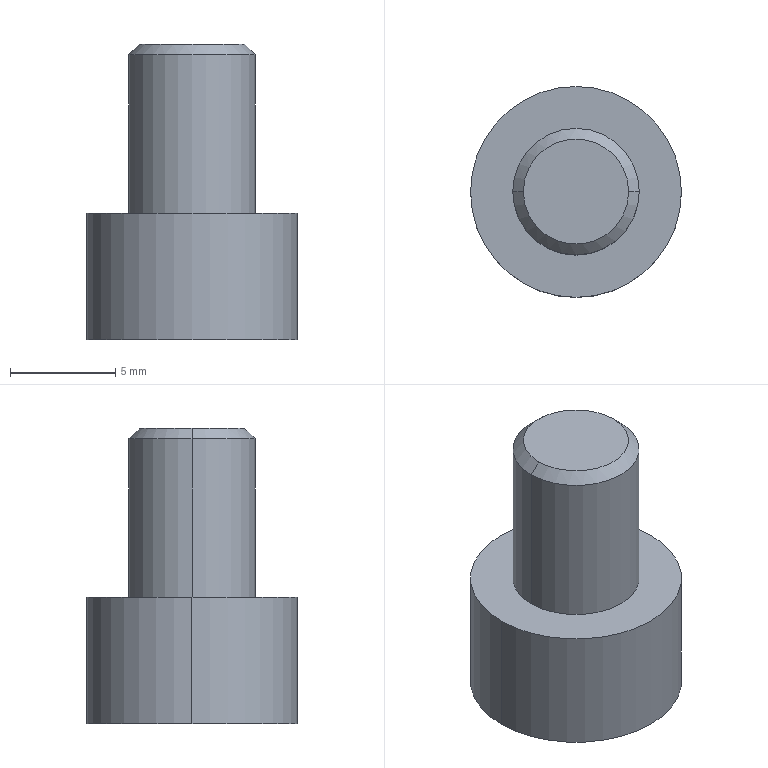Part | STEP file | M6X8 Hex Socket Screw | 1 solid | 22 faces | box 10 x 10 x 14 mm | volume 616.111 mm3 | plane 16 | cylinder 4 | cone 2 | commonest cylinder face diameters 6 x2 10 x2
STEP:
#1=CARTESIAN_POINT('',(0.,0.,0.));
#2=DIRECTION('',(0.,0.,1.));
#3=DIRECTION('',(1.,0.,0.));
#4=AXIS2_PLACEMENT_3D('',#1,#2,#3);
#5=CARTESIAN_POINT('',(2.5,0.,14.));
#6=VERTEX_POINT('',#5);
#7=CARTESIAN_POINT('',(-2.5,0.,14.));
#8=VERTEX_POINT('',#7);
#9=CARTESIAN_POINT('',(0.,0.,14.));
#10=DIRECTION('',(0.,0.,1.));
#11=DIRECTION('',(1.,0.,0.));
#12=AXIS2_PLACEMENT_3D('',#9,#10,#11);
#13=CIRCLE('',#12,2.5);
#14=CARTESIAN_POINT('',(0.,0.,14.));
#15=DIRECTION('',(0.,0.,-1.));
#16=DIRECTION('',(-1.,0.,0.));
#17=AXIS2_PLACEMENT_3D('',#14,#15,#16);
#18=CONICAL_SURFACE('',#17,2.5,0.7854);
#19=CARTESIAN_POINT('',(3.142,0.));
#20=DIRECTION('',(-1.,0.));
#21=VECTOR('',#20,1.);
#22=LINE('',#19,#21);
#23=(GEOMETRIC_REPRESENTATION_CONTEXT(2)PARAMETRIC_REPRESENTATION_CONTEXT()REPRESENTATION_CONTEXT('',''));
#24=DEFINITIONAL_REPRESENTATION('',(#22),#23);
#25=PCURVE('',#18,#24);
#26=CARTESIAN_POINT('',(3.,0.,14.));
#27=DIRECTION('',(0.,0.,1.));
#28=DIRECTION('',(1.,0.,0.));
#29=AXIS2_PLACEMENT_3D('',#26,#27,#28);
#30=PLANE('',#29);
#31=CARTESIAN_POINT('',(-3.,0.));
#32=DIRECTION('',(1.,0.));
#33=AXIS2_PLACEMENT_2D('',#31,#32);
#34=CIRCLE('',#33,2.5);
#35=(GEOMETRIC_REPRESENTATION_CONTEXT(2)PARAMETRIC_REPRESENTATION_CONTEXT()REPRESENTATION_CONTEXT('',''));
#36=DEFINITIONAL_REPRESENTATION('',(#34),#35);
#37=PCURVE('',#30,#36);
#38=SURFACE_CURVE('',#13,(#25,#37),.PCURVE_S1.);
#39=EDGE_CURVE('',#6,#8,#38,.T.);
#40=ORIENTED_EDGE('',*,*,#39,.F.);
#41=CARTESIAN_POINT('',(3.,0.,13.5));
#42=VERTEX_POINT('',#41);
#43=CARTESIAN_POINT('',(2.5,0.,14.));
#44=DIRECTION('',(0.7071,0.,-0.7071));
#45=VECTOR('',#44,1.);
#46=LINE('',#43,#45);
#47=CARTESIAN_POINT('',(3.142,0.));
#48=DIRECTION('',(0.,1.));
#49=VECTOR('',#48,1.);
#50=LINE('',#47,#49);
#51=(GEOMETRIC_REPRESENTATION_CONTEXT(2)PARAMETRIC_REPRESENTATION_CONTEXT()REPRESENTATION_CONTEXT('',''));
#52=DEFINITIONAL_REPRESENTATION('',(#50),#51);
#53=PCURVE('',#18,#52);
#54=CARTESIAN_POINT('',(0.,0.,14.));
#55=DIRECTION('',(0.,0.,-1.));
#56=DIRECTION('',(-1.,0.,0.));
#57=AXIS2_PLACEMENT_3D('',#54,#55,#56);
#58=CONICAL_SURFACE('',#57,2.5,0.7854);
#59=CARTESIAN_POINT('',(3.142,0.));
#60=DIRECTION('',(0.,1.));
#61=VECTOR('',#60,1.);
#62=LINE('',#59,#61);
#63=(GEOMETRIC_REPRESENTATION_CONTEXT(2)PARAMETRIC_REPRESENTATION_CONTEXT()REPRESENTATION_CONTEXT('',''));
#64=DEFINITIONAL_REPRESENTATION('',(#62),#63);
#65=PCURVE('',#58,#64);
#66=SURFACE_CURVE('',#46,(#53,#65),.PCURVE_S1.);
#67=EDGE_CURVE('',#6,#42,#66,.T.);
#68=ORIENTED_EDGE('',*,*,#67,.T.);
#69=CARTESIAN_POINT('',(-3.,0.,13.5));
#70=VERTEX_POINT('',#69);
#71=CARTESIAN_POINT('',(0.,0.,13.5));
#72=DIRECTION('',(0.,0.,-1.));
#73=DIRECTION('',(1.,0.,0.));
#74=AXIS2_PLACEMENT_3D('',#71,#72,#73);
#75=CIRCLE('',#74,3.);
#76=CARTESIAN_POINT('',(-3.142,0.5));
#77=DIRECTION('',(1.,0.));
#78=VECTOR('',#77,1.);
#79=LINE('',#76,#78);
#80=(GEOMETRIC_REPRESENTATION_CONTEXT(2)PARAMETRIC_REPRESENTATION_CONTEXT()REPRESENTATION_CONTEXT('',''));
#81=DEFINITIONAL_REPRESENTATION('',(#79),#80);
#82=PCURVE('',#18,#81);
#83=CARTESIAN_POINT('',(0.,0.,14.));
#84=DIRECTION('',(0.,0.,1.));
#85=DIRECTION('',(1.,0.,0.));
#86=AXIS2_PLACEMENT_3D('',#83,#84,#85);
#87=CYLINDRICAL_SURFACE('',#86,3.);
#88=CARTESIAN_POINT('',(6.283,-0.5));
#89=DIRECTION('',(-1.,0.));
#90=VECTOR('',#89,1.);
#91=LINE('',#88,#90);
#92=(GEOMETRIC_REPRESENTATION_CONTEXT(2)PARAMETRIC_REPRESENTATION_CONTEXT()REPRESENTATION_CONTEXT('',''));
#93=DEFINITIONAL_REPRESENTATION('',(#91),#92);
#94=PCURVE('',#87,#93);
#95=SURFACE_CURVE('',#75,(#82,#94),.PCURVE_S1.);
#96=EDGE_CURVE('',#70,#42,#95,.T.);
#97=ORIENTED_EDGE('',*,*,#96,.F.);
#98=CARTESIAN_POINT('',(-2.5,0.,14.));
#99=DIRECTION('',(-0.7071,0.,-0.7071));
#100=VECTOR('',#99,1.);
#101=LINE('',#98,#100);
#102=CARTESIAN_POINT('',(0.,0.));
#103=DIRECTION('',(0.,1.));
#104=VECTOR('',#103,1.);
#105=LINE('',#102,#104);
#106=(GEOMETRIC_REPRESENTATION_CONTEXT(2)PARAMETRIC_REPRESENTATION_CONTEXT()REPRESENTATION_CONTEXT('',''));
#107=DEFINITIONAL_REPRESENTATION('',(#105),#106);
#108=PCURVE('',#18,#107);
#109=CARTESIAN_POINT('',(6.283,0.));
#110=DIRECTION('',(0.,1.));
#111=VECTOR('',#110,1.);
#112=LINE('',#109,#111);
#113=(GEOMETRIC_REPRESENTATION_CONTEXT(2)PARAMETRIC_REPRESENTATION_CONTEXT()REPRESENTATION_CONTEXT('',''));
#114=DEFINITIONAL_REPRESENTATION('',(#112),#113);
#115=PCURVE('',#58,#114);
#116=SURFACE_CURVE('',#101,(#108,#115),.PCURVE_S1.);
#117=EDGE_CURVE('',#8,#70,#116,.T.);
#118=ORIENTED_EDGE('',*,*,#117,.F.);
#119=EDGE_LOOP('',(#40,#68,#97,#118));
#120=FACE_BOUND('',#119,.T.);
#121=ADVANCED_FACE('',(#120),#18,.T.);
#122=CARTESIAN_POINT('',(3.,0.,6.));
#123=VERTEX_POINT('',#122);
#124=CARTESIAN_POINT('',(-3.,0.,6.));
#125=VERTEX_POINT('',#124);
#126=CARTESIAN_POINT('',(0.,0.,6.));
#127=DIRECTION('',(0.,0.,1.));
#128=DIRECTION('',(1.,0.,0.));
#129=AXIS2_PLACEMENT_3D('',#126,#127,#128);
#130=CIRCLE('',#129,3.);
#131=CARTESIAN_POINT('',(0.,-8.));
#132=DIRECTION('',(1.,0.));
#133=VECTOR('',#132,1.);
#134=LINE('',#131,#133);
#135=(GEOMETRIC_REPRESENTATION_CONTEXT(2)PARAMETRIC_REPRESENTATION_CONTEXT()REPRESENTATION_CONTEXT('',''));
#136=DEFINITIONAL_REPRESENTATION('',(#134),#135);
#137=PCURVE('',#87,#136);
#138=CARTESIAN_POINT('',(5.,0.,6.));
#139=DIRECTION('',(0.,0.,1.));
#140=DIRECTION('',(1.,0.,0.));
#141=AXIS2_PLACEMENT_3D('',#138,#139,#140);
#142=PLANE('',#141);
#143=CARTESIAN_POINT('',(-5.,0.));
#144=DIRECTION('',(1.,0.));
#145=AXIS2_PLACEMENT_2D('',#143,#144);
#146=CIRCLE('',#145,3.);
#147=(GEOMETRIC_REPRESENTATION_CONTEXT(2)PARAMETRIC_REPRESENTATION_CONTEXT()REPRESENTATION_CONTEXT('',''));
#148=DEFINITIONAL_REPRESENTATION('',(#146),#147);
#149=PCURVE('',#142,#148);
#150=SURFACE_CURVE('',#130,(#137,#149),.PCURVE_S1.);
#151=EDGE_CURVE('',#123,#125,#150,.T.);
#152=ORIENTED_EDGE('',*,*,#151,.T.);
#153=CARTESIAN_POINT('',(-3.,0.,14.));
#154=DIRECTION('',(0.,0.,1.));
#155=VECTOR('',#154,1.);
#156=LINE('',#153,#155);
#157=CARTESIAN_POINT('',(3.142,0.));
#158=DIRECTION('',(0.,1.));
#159=VECTOR('',#158,1.);
#160=LINE('',#157,#159);
#161=(GEOMETRIC_REPRESENTATION_CONTEXT(2)PARAMETRIC_REPRESENTATION_CONTEXT()REPRESENTATION_CONTEXT('',''));
#162=DEFINITIONAL_REPRESENTATION('',(#160),#161);
#163=PCURVE('',#87,#162);
#164=CARTESIAN_POINT('',(0.,0.,14.));
#165=DIRECTION('',(0.,0.,1.));
#166=DIRECTION('',(1.,0.,0.));
#167=AXIS2_PLACEMENT_3D('',#164,#165,#166);
#168=CYLINDRICAL_SURFACE('',#167,3.);
#169=CARTESIAN_POINT('',(3.142,0.));
#170=DIRECTION('',(0.,1.));
#171=VECTOR('',#170,1.);
#172=LINE('',#169,#171);
#173=(GEOMETRIC_REPRESENTATION_CONTEXT(2)PARAMETRIC_REPRESENTATION_CONTEXT()REPRESENTATION_CONTEXT('',''));
#174=DEFINITIONAL_REPRESENTATION('',(#172),#173);
#175=PCURVE('',#168,#174);
#176=SURFACE_CURVE('',#156,(#163,#175),.PCURVE_S1.);
#177=EDGE_CURVE('',#125,#70,#176,.T.);
#178=ORIENTED_EDGE('',*,*,#177,.T.);
#179=ORIENTED_EDGE('',*,*,#96,.T.);
#180=CARTESIAN_POINT('',(3.,0.,14.));
#181=DIRECTION('',(0.,0.,1.));
#182=VECTOR('',#181,1.);
#183=LINE('',#180,#182);
#184=CARTESIAN_POINT('',(0.,0.));
#185=DIRECTION('',(0.,1.));
#186=VECTOR('',#185,1.);
#187=LINE('',#184,#186);
#188=(GEOMETRIC_REPRESENTATION_CONTEXT(2)PARAMETRIC_REPRESENTATION_CONTEXT()REPRESENTATION_CONTEXT('',''));
#189=DEFINITIONAL_REPRESENTATION('',(#187),#188);
#190=PCURVE('',#87,#189);
#191=CARTESIAN_POINT('',(6.283,0.));
#192=DIRECTION('',(0.,1.));
#193=VECTOR('',#192,1.);
#194=LINE('',#191,#193);
#195=(GEOMETRIC_REPRESENTATION_CONTEXT(2)PARAMETRIC_REPRESENTATION_CONTEXT()REPRESENTATION_CONTEXT('',''));
#196=DEFINITIONAL_REPRESENTATION('',(#194),#195);
#197=PCURVE('',#168,#196);
#198=SURFACE_CURVE('',#183,(#190,#197),.PCURVE_S1.);
#199=EDGE_CURVE('',#123,#42,#198,.T.);
#200=ORIENTED_EDGE('',*,*,#199,.F.);
#201=EDGE_LOOP('',(#152,#178,#179,#200));
#202=FACE_BOUND('',#201,.T.);
#203=ADVANCED_FACE('',(#202),#87,.T.);
#204=CARTESIAN_POINT('',(5.,0.,0.));
#205=VERTEX_POINT('',#204);
#206=CARTESIAN_POINT('',(-5.,0.,0.));
#207=VERTEX_POINT('',#206);
#208=CARTESIAN_POINT('',(0.,0.,0.));
#209=DIRECTION('',(0.,0.,1.));
#210=DIRECTION('',(1.,0.,0.));
#211=AXIS2_PLACEMENT_3D('',#208,#209,#210);
#212=CIRCLE('',#211,5.);
#213=CARTESIAN_POINT('',(0.,0.,14.));
#214=DIRECTION('',(0.,0.,1.));
#215=DIRECTION('',(1.,0.,0.));
#216=AXIS2_PLACEMENT_3D('',#213,#214,#215);
#217=CYLINDRICAL_SURFACE('',#216,5.);
#218=CARTESIAN_POINT('',(0.,-14.));
#219=DIRECTION('',(1.,0.));
#220=VECTOR('',#219,1.);
#221=LINE('',#218,#220);
#222=(GEOMETRIC_REPRESENTATION_CONTEXT(2)PARAMETRIC_REPRESENTATION_CONTEXT()REPRESENTATION_CONTEXT('',''));
#223=DEFINITIONAL_REPRESENTATION('',(#221),#222);
#224=PCURVE('',#217,#223);
#225=CARTESIAN_POINT('',(0.,0.,0.));
#226=DIRECTION('',(0.,0.,-1.));
#227=DIRECTION('',(-1.,0.,0.));
#228=AXIS2_PLACEMENT_3D('',#225,#226,#227);
#229=PLANE('',#228);
#230=CARTESIAN_POINT('',(-5.,0.));
#231=CARTESIAN_POINT('',(-5.,8.66));
#232=CARTESIAN_POINT('',(2.5,4.33));
#233=CARTESIAN_POINT('',(10.,0.));
#234=CARTESIAN_POINT('',(2.5,-4.33));
#235=CARTESIAN_POINT('',(-5.,-8.66));
#236=CARTESIAN_POINT('',(-5.,0.));
#237=(BOUNDED_CURVE()B_SPLINE_CURVE(2,(#230,#231,#232,#233,#234,#235,#236),.UNSPECIFIED.,.T.,.F.)B_SPLINE_CURVE_WITH_KNOTS((1,2,2,2,2,1),(-2.094,0.,2.094,4.189,6.283,8.378),.UNSPECIFIED.)CURVE()GEOMETRIC_REPRESENTATION_ITEM()RATIONAL_B_SPLINE_CURVE((1.,0.5,1.,0.5,1.,0.5,1.))REPRESENTATION_ITEM(''));
#238=(GEOMETRIC_REPRESENTATION_CONTEXT(2)PARAMETRIC_REPRESENTATION_CONTEXT()REPRESENTATION_CONTEXT('',''));
#239=DEFINITIONAL_REPRESENTATION('',(#237),#238);
#240=PCURVE('',#229,#239);
#241=SURFACE_CURVE('',#212,(#224,#240),.PCURVE_S1.);
#242=EDGE_CURVE('',#205,#207,#241,.T.);
#243=ORIENTED_EDGE('',*,*,#242,.T.);
#244=CARTESIAN_POINT('',(-5.,0.,6.));
#245=VERTEX_POINT('',#244);
#246=CARTESIAN_POINT('',(-5.,0.,14.));
#247=DIRECTION('',(0.,0.,1.));
#248=VECTOR('',#247,1.);
#249=LINE('',#246,#248);
#250=CARTESIAN_POINT('',(3.142,0.));
#251=DIRECTION('',(0.,1.));
#252=VECTOR('',#251,1.);
#253=LINE('',#250,#252);
#254=(GEOMETRIC_REPRESENTATION_CONTEXT(2)PARAMETRIC_REPRESENTATION_CONTEXT()REPRESENTATION_CONTEXT('',''));
#255=DEFINITIONAL_REPRESENTATION('',(#253),#254);
#256=PCURVE('',#217,#255);
#257=CARTESIAN_POINT('',(0.,0.,14.));
#258=DIRECTION('',(0.,0.,1.));
#259=DIRECTION('',(1.,0.,0.));
#260=AXIS2_PLACEMENT_3D('',#257,#258,#259);
#261=CYLINDRICAL_SURFACE('',#260,5.);
#262=CARTESIAN_POINT('',(3.142,0.));
#263=DIRECTION('',(0.,1.));
#264=VECTOR('',#263,1.);
#265=LINE('',#262,#264);
#266=(GEOMETRIC_REPRESENTATION_CONTEXT(2)PARAMETRIC_REPRESENTATION_CONTEXT()REPRESENTATION_CONTEXT('',''));
#267=DEFINITIONAL_REPRESENTATION('',(#265),#266);
#268=PCURVE('',#261,#267);
#269=SURFACE_CURVE('',#249,(#256,#268),.PCURVE_S1.);
#270=EDGE_CURVE('',#207,#245,#269,.T.);
#271=ORIENTED_EDGE('',*,*,#270,.T.);
#272=CARTESIAN_POINT('',(5.,0.,6.));
#273=VERTEX_POINT('',#272);
#274=CARTESIAN_POINT('',(0.,0.,6.));
#275=DIRECTION('',(0.,0.,1.));
#276=DIRECTION('',(1.,0.,0.));
#277=AXIS2_PLACEMENT_3D('',#274,#275,#276);
#278=CIRCLE('',#277,5.);
#279=CARTESIAN_POINT('',(0.,-8.));
#280=DIRECTION('',(1.,0.));
#281=VECTOR('',#280,1.);
#282=LINE('',#279,#281);
#283=(GEOMETRIC_REPRESENTATION_CONTEXT(2)PARAMETRIC_REPRESENTATION_CONTEXT()REPRESENTATION_CONTEXT('',''));
#284=DEFINITIONAL_REPRESENTATION('',(#282),#283);
#285=PCURVE('',#217,#284);
#286=CARTESIAN_POINT('',(-5.,0.));
#287=DIRECTION('',(1.,0.));
#288=AXIS2_PLACEMENT_2D('',#286,#287);
#289=CIRCLE('',#288,5.);
#290=(GEOMETRIC_REPRESENTATION_CONTEXT(2)PARAMETRIC_REPRESENTATION_CONTEXT()REPRESENTATION_CONTEXT('',''));
#291=DEFINITIONAL_REPRESENTATION('',(#289),#290);
#292=PCURVE('',#142,#291);
#293=SURFACE_CURVE('',#278,(#285,#292),.PCURVE_S1.);
#294=EDGE_CURVE('',#273,#245,#293,.T.);
#295=ORIENTED_EDGE('',*,*,#294,.F.);
#296=CARTESIAN_POINT('',(5.,0.,14.));
#297=DIRECTION('',(0.,0.,1.));
#298=VECTOR('',#297,1.);
#299=LINE('',#296,#298);
#300=CARTESIAN_POINT('',(0.,0.));
#301=DIRECTION('',(0.,1.));
#302=VECTOR('',#301,1.);
#303=LINE('',#300,#302);
#304=(GEOMETRIC_REPRESENTATION_CONTEXT(2)PARAMETRIC_REPRESENTATION_CONTEXT()REPRESENTATION_CONTEXT('',''));
#305=DEFINITIONAL_REPRESENTATION('',(#303),#304);
#306=PCURVE('',#217,#305);
#307=CARTESIAN_POINT('',(6.283,0.));
#308=DIRECTION('',(0.,1.));
#309=VECTOR('',#308,1.);
#310=LINE('',#307,#309);
#311=(GEOMETRIC_REPRESENTATION_CONTEXT(2)PARAMETRIC_REPRESENTATION_CONTEXT()REPRESENTATION_CONTEXT('',''));
#312=DEFINITIONAL_REPRESENTATION('',(#310),#311);
#313=PCURVE('',#261,#312);
#314=SURFACE_CURVE('',#299,(#306,#313),.PCURVE_S1.);
#315=EDGE_CURVE('',#205,#273,#314,.T.);
#316=ORIENTED_EDGE('',*,*,#315,.F.);
#317=EDGE_LOOP('',(#243,#271,#295,#316));
#318=FACE_BOUND('',#317,.T.);
#319=ADVANCED_FACE('',(#318),#217,.T.);
#320=CARTESIAN_POINT('',(1.443,-2.5,0.));
#321=VERTEX_POINT('',#320);
#322=CARTESIAN_POINT('',(-1.443,-2.5,0.));
#323=VERTEX_POINT('',#322);
#324=CARTESIAN_POINT('',(1.443,-2.5,0.));
#325=DIRECTION('',(-1.,0.,0.));
#326=VECTOR('',#325,1.);
#327=LINE('',#324,#326);
#328=CARTESIAN_POINT('',(-1.443,-2.5));
#329=DIRECTION('',(1.,0.));
#330=VECTOR('',#329,1.);
#331=LINE('',#328,#330);
#332=(GEOMETRIC_REPRESENTATION_CONTEXT(2)PARAMETRIC_REPRESENTATION_CONTEXT()REPRESENTATION_CONTEXT('',''));
#333=DEFINITIONAL_REPRESENTATION('',(#331),#332);
#334=PCURVE('',#229,#333);
#335=CARTESIAN_POINT('',(1.443,-2.5,4.));
#336=DIRECTION('',(0.,-1.,0.));
#337=DIRECTION('',(1.,0.,0.));
#338=AXIS2_PLACEMENT_3D('',#335,#336,#337);
#339=PLANE('',#338);
#340=CARTESIAN_POINT('',(0.,-4.));
#341=DIRECTION('',(-1.,0.));
#342=VECTOR('',#341,1.);
#343=LINE('',#340,#342);
#344=(GEOMETRIC_REPRESENTATION_CONTEXT(2)PARAMETRIC_REPRESENTATION_CONTEXT()REPRESENTATION_CONTEXT('',''));
#345=DEFINITIONAL_REPRESENTATION('',(#343),#344);
#346=PCURVE('',#339,#345);
#347=SURFACE_CURVE('',#327,(#334,#346),.PCURVE_S1.);
#348=EDGE_CURVE('',#321,#323,#347,.T.);
#349=ORIENTED_EDGE('',*,*,#348,.F.);
#350=CARTESIAN_POINT('',(2.887,0.,0.));
#351=VERTEX_POINT('',#350);
#352=CARTESIAN_POINT('',(2.887,0.,0.));
#353=DIRECTION('',(-0.5,-0.866,0.));
#354=VECTOR('',#353,1.);
#355=LINE('',#352,#354);
#356=CARTESIAN_POINT('',(-2.887,0.));
#357=DIRECTION('',(0.5,-0.866));
#358=VECTOR('',#357,1.);
#359=LINE('',#356,#358);
#360=(GEOMETRIC_REPRESENTATION_CONTEXT(2)PARAMETRIC_REPRESENTATION_CONTEXT()REPRESENTATION_CONTEXT('',''));
#361=DEFINITIONAL_REPRESENTATION('',(#359),#360);
#362=PCURVE('',#229,#361);
#363=CARTESIAN_POINT('',(2.887,0.,4.));
#364=DIRECTION('',(0.866,-0.5,0.));
#365=DIRECTION('',(0.5,0.866,0.));
#366=AXIS2_PLACEMENT_3D('',#363,#364,#365);
#367=PLANE('',#366);
#368=CARTESIAN_POINT('',(0.,-4.));
#369=DIRECTION('',(-1.,0.));
#370=VECTOR('',#369,1.);
#371=LINE('',#368,#370);
#372=(GEOMETRIC_REPRESENTATION_CONTEXT(2)PARAMETRIC_REPRESENTATION_CONTEXT()REPRESENTATION_CONTEXT('',''));
#373=DEFINITIONAL_REPRESENTATION('',(#371),#372);
#374=PCURVE('',#367,#373);
#375=SURFACE_CURVE('',#355,(#362,#374),.PCURVE_S1.);
#376=EDGE_CURVE('',#351,#321,#375,.T.);
#377=ORIENTED_EDGE('',*,*,#376,.F.);
#378=CARTESIAN_POINT('',(1.443,2.5,0.));
#379=VERTEX_POINT('',#378);
#380=CARTESIAN_POINT('',(1.443,2.5,0.));
#381=DIRECTION('',(0.5,-0.866,0.));
#382=VECTOR('',#381,1.);
#383=LINE('',#380,#382);
#384=CARTESIAN_POINT('',(-1.443,2.5));
#385=DIRECTION('',(-0.5,-0.866));
#386=VECTOR('',#385,1.);
#387=LINE('',#384,#386);
#388=(GEOMETRIC_REPRESENTATION_CONTEXT(2)PARAMETRIC_REPRESENTATION_CONTEXT()REPRESENTATION_CONTEXT('',''));
#389=DEFINITIONAL_REPRESENTATION('',(#387),#388);
#390=PCURVE('',#229,#389);
#391=CARTESIAN_POINT('',(1.443,2.5,4.));
#392=DIRECTION('',(0.866,0.5,0.));
#393=DIRECTION('',(-0.5,0.866,0.));
#394=AXIS2_PLACEMENT_3D('',#391,#392,#393);
#395=PLANE('',#394);
#396=CARTESIAN_POINT('',(0.,-4.));
#397=DIRECTION('',(-1.,0.));
#398=VECTOR('',#397,1.);
#399=LINE('',#396,#398);
#400=(GEOMETRIC_REPRESENTATION_CONTEXT(2)PARAMETRIC_REPRESENTATION_CONTEXT()REPRESENTATION_CONTEXT('',''));
#401=DEFINITIONAL_REPRESENTATION('',(#399),#400);
#402=PCURVE('',#395,#401);
#403=SURFACE_CURVE('',#383,(#390,#402),.PCURVE_S1.);
#404=EDGE_CURVE('',#379,#351,#403,.T.);
#405=ORIENTED_EDGE('',*,*,#404,.F.);
#406=CARTESIAN_POINT('',(-1.443,2.5,0.));
#407=VERTEX_POINT('',#406);
#408=CARTESIAN_POINT('',(-1.443,2.5,0.));
#409=DIRECTION('',(1.,0.,0.));
#410=VECTOR('',#409,1.);
#411=LINE('',#408,#410);
#412=CARTESIAN_POINT('',(1.443,2.5));
#413=DIRECTION('',(-1.,0.));
#414=VECTOR('',#413,1.);
#415=LINE('',#412,#414);
#416=(GEOMETRIC_REPRESENTATION_CONTEXT(2)PARAMETRIC_REPRESENTATION_CONTEXT()REPRESENTATION_CONTEXT('',''));
#417=DEFINITIONAL_REPRESENTATION('',(#415),#416);
#418=PCURVE('',#229,#417);
#419=CARTESIAN_POINT('',(-1.443,2.5,4.));
#420=DIRECTION('',(0.,1.,0.));
#421=DIRECTION('',(-1.,0.,0.));
#422=AXIS2_PLACEMENT_3D('',#419,#420,#421);
#423=PLANE('',#422);
#424=CARTESIAN_POINT('',(0.,-4.));
#425=DIRECTION('',(-1.,0.));
#426=VECTOR('',#425,1.);
#427=LINE('',#424,#426);
#428=(GEOMETRIC_REPRESENTATION_CONTEXT(2)PARAMETRIC_REPRESENTATION_CONTEXT()REPRESENTATION_CONTEXT('',''));
#429=DEFINITIONAL_REPRESENTATION('',(#427),#428);
#430=PCURVE('',#423,#429);
#431=SURFACE_CURVE('',#411,(#418,#430),.PCURVE_S1.);
#432=EDGE_CURVE('',#407,#379,#431,.T.);
#433=ORIENTED_EDGE('',*,*,#432,.F.);
#434=CARTESIAN_POINT('',(-2.887,0.,0.));
#435=VERTEX_POINT('',#434);
#436=CARTESIAN_POINT('',(-2.887,0.,0.));
#437=DIRECTION('',(0.5,0.866,0.));
#438=VECTOR('',#437,1.);
#439=LINE('',#436,#438);
#440=CARTESIAN_POINT('',(2.887,0.));
#441=DIRECTION('',(-0.5,0.866));
#442=VECTOR('',#441,1.);
#443=LINE('',#440,#442);
#444=(GEOMETRIC_REPRESENTATION_CONTEXT(2)PARAMETRIC_REPRESENTATION_CONTEXT()REPRESENTATION_CONTEXT('',''));
#445=DEFINITIONAL_REPRESENTATION('',(#443),#444);
#446=PCURVE('',#229,#445);
#447=CARTESIAN_POINT('',(-2.887,0.,4.));
#448=DIRECTION('',(-0.866,0.5,0.));
#449=DIRECTION('',(-0.5,-0.866,0.));
#450=AXIS2_PLACEMENT_3D('',#447,#448,#449);
#451=PLANE('',#450);
#452=CARTESIAN_POINT('',(0.,-4.));
#453=DIRECTION('',(-1.,0.));
#454=VECTOR('',#453,1.);
#455=LINE('',#452,#454);
#456=(GEOMETRIC_REPRESENTATION_CONTEXT(2)PARAMETRIC_REPRESENTATION_CONTEXT()REPRESENTATION_CONTEXT('',''));
#457=DEFINITIONAL_REPRESENTATION('',(#455),#456);
#458=PCURVE('',#451,#457);
#459=SURFACE_CURVE('',#439,(#446,#458),.PCURVE_S1.);
#460=EDGE_CURVE('',#435,#407,#459,.T.);
#461=ORIENTED_EDGE('',*,*,#460,.F.);
#462=CARTESIAN_POINT('',(-1.443,-2.5,0.));
#463=DIRECTION('',(-0.5,0.866,0.));
#464=VECTOR('',#463,1.);
#465=LINE('',#462,#464);
#466=CARTESIAN_POINT('',(1.443,-2.5));
#467=DIRECTION('',(0.5,0.866));
#468=VECTOR('',#467,1.);
#469=LINE('',#466,#468);
#470=(GEOMETRIC_REPRESENTATION_CONTEXT(2)PARAMETRIC_REPRESENTATION_CONTEXT()REPRESENTATION_CONTEXT('',''));
#471=DEFINITIONAL_REPRESENTATION('',(#469),#470);
#472=PCURVE('',#229,#471);
#473=CARTESIAN_POINT('',(-1.443,-2.5,4.));
#474=DIRECTION('',(-0.866,-0.5,0.));
#475=DIRECTION('',(0.5,-0.866,0.));
#476=AXIS2_PLACEMENT_3D('',#473,#474,#475);
#477=PLANE('',#476);
#478=CARTESIAN_POINT('',(0.,-4.));
#479=DIRECTION('',(-1.,0.));
#480=VECTOR('',#479,1.);
#481=LINE('',#478,#480);
#482=(GEOMETRIC_REPRESENTATION_CONTEXT(2)PARAMETRIC_REPRESENTATION_CONTEXT()REPRESENTATION_CONTEXT('',''));
#483=DEFINITIONAL_REPRESENTATION('',(#481),#482);
#484=PCURVE('',#477,#483);
#485=SURFACE_CURVE('',#465,(#472,#484),.PCURVE_S1.);
#486=EDGE_CURVE('',#323,#435,#485,.T.);
#487=ORIENTED_EDGE('',*,*,#486,.F.);
#488=EDGE_LOOP('',(#349,#377,#405,#433,#461,#487));
#489=FACE_BOUND('',#488,.T.);
#490=ORIENTED_EDGE('',*,*,#242,.F.);
#491=CARTESIAN_POINT('',(0.,0.,0.));
#492=DIRECTION('',(0.,0.,1.));
#493=DIRECTION('',(1.,0.,0.));
#494=AXIS2_PLACEMENT_3D('',#491,#492,#493);
#495=CIRCLE('',#494,5.);
#496=CARTESIAN_POINT('',(-5.,0.));
#497=CARTESIAN_POINT('',(-5.,8.66));
#498=CARTESIAN_POINT('',(2.5,4.33));
#499=CARTESIAN_POINT('',(10.,0.));
#500=CARTESIAN_POINT('',(2.5,-4.33));
#501=CARTESIAN_POINT('',(-5.,-8.66));
#502=CARTESIAN_POINT('',(-5.,0.));
#503=(BOUNDED_CURVE()B_SPLINE_CURVE(2,(#496,#497,#498,#499,#500,#501,#502),.UNSPECIFIED.,.T.,.F.)B_SPLINE_CURVE_WITH_KNOTS((1,2,2,2,2,1),(-2.094,0.,2.094,4.189,6.283,8.378),.UNSPECIFIED.)CURVE()GEOMETRIC_REPRESENTATION_ITEM()RATIONAL_B_SPLINE_CURVE((1.,0.5,1.,0.5,1.,0.5,1.))REPRESENTATION_ITEM(''));
#504=(GEOMETRIC_REPRESENTATION_CONTEXT(2)PARAMETRIC_REPRESENTATION_CONTEXT()REPRESENTATION_CONTEXT('',''));
#505=DEFINITIONAL_REPRESENTATION('',(#503),#504);
#506=PCURVE('',#229,#505);
#507=CARTESIAN_POINT('',(0.,-14.));
#508=DIRECTION('',(1.,0.));
#509=VECTOR('',#508,1.);
#510=LINE('',#507,#509);
#511=(GEOMETRIC_REPRESENTATION_CONTEXT(2)PARAMETRIC_REPRESENTATION_CONTEXT()REPRESENTATION_CONTEXT('',''));
#512=DEFINITIONAL_REPRESENTATION('',(#510),#511);
#513=PCURVE('',#261,#512);
#514=SURFACE_CURVE('',#495,(#506,#513),.PCURVE_S1.);
#515=EDGE_CURVE('',#207,#205,#514,.T.);
#516=ORIENTED_EDGE('',*,*,#515,.F.);
#517=EDGE_LOOP('',(#490,#516));
#518=FACE_BOUND('',#517,.T.);
#519=ADVANCED_FACE('',(#489,#518),#229,.T.);
#520=ORIENTED_EDGE('',*,*,#270,.F.);
#521=ORIENTED_EDGE('',*,*,#515,.T.);
#522=ORIENTED_EDGE('',*,*,#315,.T.);
#523=CARTESIAN_POINT('',(0.,0.,6.));
#524=DIRECTION('',(0.,0.,1.));
#525=DIRECTION('',(1.,0.,0.));
#526=AXIS2_PLACEMENT_3D('',#523,#524,#525);
#527=CIRCLE('',#526,5.);
#528=CARTESIAN_POINT('',(0.,-8.));
#529=DIRECTION('',(1.,0.));
#530=VECTOR('',#529,1.);
#531=LINE('',#528,#530);
#532=(GEOMETRIC_REPRESENTATION_CONTEXT(2)PARAMETRIC_REPRESENTATION_CONTEXT()REPRESENTATION_CONTEXT('',''));
#533=DEFINITIONAL_REPRESENTATION('',(#531),#532);
#534=PCURVE('',#261,#533);
#535=CARTESIAN_POINT('',(-5.,0.));
#536=DIRECTION('',(1.,0.));
#537=AXIS2_PLACEMENT_2D('',#535,#536);
#538=CIRCLE('',#537,5.);
#539=(GEOMETRIC_REPRESENTATION_CONTEXT(2)PARAMETRIC_REPRESENTATION_CONTEXT()REPRESENTATION_CONTEXT('',''));
#540=DEFINITIONAL_REPRESENTATION('',(#538),#539);
#541=PCURVE('',#142,#540);
#542=SURFACE_CURVE('',#527,(#534,#541),.PCURVE_S1.);
#543=EDGE_CURVE('',#245,#273,#542,.T.);
#544=ORIENTED_EDGE('',*,*,#543,.F.);
#545=EDGE_LOOP('',(#520,#521,#522,#544));
#546=FACE_BOUND('',#545,.T.);
#547=ADVANCED_FACE('',(#546),#261,.T.);
#548=ORIENTED_EDGE('',*,*,#294,.T.);
#549=ORIENTED_EDGE('',*,*,#543,.T.);
#550=EDGE_LOOP('',(#548,#549));
#551=FACE_BOUND('',#550,.T.);
#552=ORIENTED_EDGE('',*,*,#151,.F.);
#553=CARTESIAN_POINT('',(0.,0.,6.));
#554=DIRECTION('',(0.,0.,1.));
#555=DIRECTION('',(1.,0.,0.));
#556=AXIS2_PLACEMENT_3D('',#553,#554,#555);
#557=CIRCLE('',#556,3.);
#558=CARTESIAN_POINT('',(-5.,0.));
#559=DIRECTION('',(1.,0.));
#560=AXIS2_PLACEMENT_2D('',#558,#559);
#561=CIRCLE('',#560,3.);
#562=(GEOMETRIC_REPRESENTATION_CONTEXT(2)PARAMETRIC_REPRESENTATION_CONTEXT()REPRESENTATION_CONTEXT('',''));
#563=DEFINITIONAL_REPRESENTATION('',(#561),#562);
#564=PCURVE('',#142,#563);
#565=CARTESIAN_POINT('',(0.,-8.));
#566=DIRECTION('',(1.,0.));
#567=VECTOR('',#566,1.);
#568=LINE('',#565,#567);
#569=(GEOMETRIC_REPRESENTATION_CONTEXT(2)PARAMETRIC_REPRESENTATION_CONTEXT()REPRESENTATION_CONTEXT('',''));
#570=DEFINITIONAL_REPRESENTATION('',(#568),#569);
#571=PCURVE('',#168,#570);
#572=SURFACE_CURVE('',#557,(#564,#571),.PCURVE_S1.);
#573=EDGE_CURVE('',#125,#123,#572,.T.);
#574=ORIENTED_EDGE('',*,*,#573,.F.);
#575=EDGE_LOOP('',(#552,#574));
#576=FACE_BOUND('',#575,.T.);
#577=ADVANCED_FACE('',(#551,#576),#142,.T.);
#578=ORIENTED_EDGE('',*,*,#177,.F.);
#579=ORIENTED_EDGE('',*,*,#573,.T.);
#580=ORIENTED_EDGE('',*,*,#199,.T.);
#581=CARTESIAN_POINT('',(0.,0.,13.5));
#582=DIRECTION('',(0.,0.,-1.));
#583=DIRECTION('',(1.,0.,0.));
#584=AXIS2_PLACEMENT_3D('',#581,#582,#583);
#585=CIRCLE('',#584,3.);
#586=CARTESIAN_POINT('',(6.283,-0.5));
#587=DIRECTION('',(-1.,0.));
#588=VECTOR('',#587,1.);
#589=LINE('',#586,#588);
#590=(GEOMETRIC_REPRESENTATION_CONTEXT(2)PARAMETRIC_REPRESENTATION_CONTEXT()REPRESENTATION_CONTEXT('',''));
#591=DEFINITIONAL_REPRESENTATION('',(#589),#590);
#592=PCURVE('',#168,#591);
#593=CARTESIAN_POINT('',(3.142,0.5));
#594=DIRECTION('',(1.,0.));
#595=VECTOR('',#594,1.);
#596=LINE('',#593,#595);
#597=(GEOMETRIC_REPRESENTATION_CONTEXT(2)PARAMETRIC_REPRESENTATION_CONTEXT()REPRESENTATION_CONTEXT('',''));
#598=DEFINITIONAL_REPRESENTATION('',(#596),#597);
#599=PCURVE('',#58,#598);
#600=SURFACE_CURVE('',#585,(#592,#599),.PCURVE_S1.);
#601=EDGE_CURVE('',#42,#70,#600,.T.);
#602=ORIENTED_EDGE('',*,*,#601,.T.);
#603=EDGE_LOOP('',(#578,#579,#580,#602));
#604=FACE_BOUND('',#603,.T.);
#605=ADVANCED_FACE('',(#604),#168,.T.);
#606=CARTESIAN_POINT('',(0.,0.,14.));
#607=DIRECTION('',(0.,0.,1.));
#608=DIRECTION('',(1.,0.,0.));
#609=AXIS2_PLACEMENT_3D('',#606,#607,#608);
#610=CIRCLE('',#609,2.5);
#611=CARTESIAN_POINT('',(-3.,0.));
#612=DIRECTION('',(1.,0.));
#613=AXIS2_PLACEMENT_2D('',#611,#612);
#614=CIRCLE('',#613,2.5);
#615=(GEOMETRIC_REPRESENTATION_CONTEXT(2)PARAMETRIC_REPRESENTATION_CONTEXT()REPRESENTATION_CONTEXT('',''));
#616=DEFINITIONAL_REPRESENTATION('',(#614),#615);
#617=PCURVE('',#30,#616);
#618=CARTESIAN_POINT('',(9.425,0.));
#619=DIRECTION('',(-1.,0.));
#620=VECTOR('',#619,1.);
#621=LINE('',#618,#620);
#622=(GEOMETRIC_REPRESENTATION_CONTEXT(2)PARAMETRIC_REPRESENTATION_CONTEXT()REPRESENTATION_CONTEXT('',''));
#623=DEFINITIONAL_REPRESENTATION('',(#621),#622);
#624=PCURVE('',#58,#623);
#625=SURFACE_CURVE('',#610,(#617,#624),.PCURVE_S1.);
#626=EDGE_CURVE('',#8,#6,#625,.T.);
#627=ORIENTED_EDGE('',*,*,#626,.T.);
#628=ORIENTED_EDGE('',*,*,#39,.T.);
#629=EDGE_LOOP('',(#627,#628));
#630=FACE_BOUND('',#629,.T.);
#631=ADVANCED_FACE('',(#630),#30,.T.);
#632=CARTESIAN_POINT('',(-1.443,-2.5,3.));
#633=VERTEX_POINT('',#632);
#634=CARTESIAN_POINT('',(-1.443,-2.5,4.));
#635=DIRECTION('',(0.,0.,-1.));
#636=VECTOR('',#635,1.);
#637=LINE('',#634,#636);
#638=CARTESIAN_POINT('',(-2.887,0.));
#639=DIRECTION('',(0.,-1.));
#640=VECTOR('',#639,1.);
#641=LINE('',#638,#640);
#642=(GEOMETRIC_REPRESENTATION_CONTEXT(2)PARAMETRIC_REPRESENTATION_CONTEXT()REPRESENTATION_CONTEXT('',''));
#643=DEFINITIONAL_REPRESENTATION('',(#641),#642);
#644=PCURVE('',#339,#643);
#645=CARTESIAN_POINT('',(0.,0.));
#646=DIRECTION('',(0.,-1.));
#647=VECTOR('',#646,1.);
#648=LINE('',#645,#647);
#649=(GEOMETRIC_REPRESENTATION_CONTEXT(2)PARAMETRIC_REPRESENTATION_CONTEXT()REPRESENTATION_CONTEXT('',''));
#650=DEFINITIONAL_REPRESENTATION('',(#648),#649);
#651=PCURVE('',#477,#650);
#652=SURFACE_CURVE('',#637,(#644,#651),.PCURVE_S1.);
#653=EDGE_CURVE('',#633,#323,#652,.T.);
#654=ORIENTED_EDGE('',*,*,#653,.F.);
#655=CARTESIAN_POINT('',(1.443,-2.5,3.));
#656=VERTEX_POINT('',#655);
#657=CARTESIAN_POINT('',(1.443,-2.5,3.));
#658=DIRECTION('',(1.,0.,0.));
#659=VECTOR('',#658,1.);
#660=LINE('',#657,#659);
#661=CARTESIAN_POINT('',(0.,-1.));
#662=DIRECTION('',(1.,0.));
#663=VECTOR('',#662,1.);
#664=LINE('',#661,#663);
#665=(GEOMETRIC_REPRESENTATION_CONTEXT(2)PARAMETRIC_REPRESENTATION_CONTEXT()REPRESENTATION_CONTEXT('',''));
#666=DEFINITIONAL_REPRESENTATION('',(#664),#665);
#667=PCURVE('',#339,#666);
#668=CARTESIAN_POINT('',(0.,-1.5,4.));
#669=DIRECTION('',(0.,-0.7071,0.7071));
#670=DIRECTION('',(-1.,0.,0.));
#671=AXIS2_PLACEMENT_3D('',#668,#669,#670);
#672=PLANE('',#671);
#673=CARTESIAN_POINT('',(-1.443,1.414));
#674=DIRECTION('',(-1.,0.));
#675=VECTOR('',#674,1.);
#676=LINE('',#673,#675);
#677=(GEOMETRIC_REPRESENTATION_CONTEXT(2)PARAMETRIC_REPRESENTATION_CONTEXT()REPRESENTATION_CONTEXT('',''));
#678=DEFINITIONAL_REPRESENTATION('',(#676),#677);
#679=PCURVE('',#672,#678);
#680=SURFACE_CURVE('',#660,(#667,#679),.PCURVE_S1.);
#681=EDGE_CURVE('',#633,#656,#680,.T.);
#682=ORIENTED_EDGE('',*,*,#681,.T.);
#683=CARTESIAN_POINT('',(1.443,-2.5,4.));
#684=DIRECTION('',(0.,0.,-1.));
#685=VECTOR('',#684,1.);
#686=LINE('',#683,#685);
#687=CARTESIAN_POINT('',(0.,0.));
#688=DIRECTION('',(0.,-1.));
#689=VECTOR('',#688,1.);
#690=LINE('',#687,#689);
#691=(GEOMETRIC_REPRESENTATION_CONTEXT(2)PARAMETRIC_REPRESENTATION_CONTEXT()REPRESENTATION_CONTEXT('',''));
#692=DEFINITIONAL_REPRESENTATION('',(#690),#691);
#693=PCURVE('',#339,#692);
#694=CARTESIAN_POINT('',(-2.887,0.));
#695=DIRECTION('',(0.,-1.));
#696=VECTOR('',#695,1.);
#697=LINE('',#694,#696);
#698=(GEOMETRIC_REPRESENTATION_CONTEXT(2)PARAMETRIC_REPRESENTATION_CONTEXT()REPRESENTATION_CONTEXT('',''));
#699=DEFINITIONAL_REPRESENTATION('',(#697),#698);
#700=PCURVE('',#367,#699);
#701=SURFACE_CURVE('',#686,(#693,#700),.PCURVE_S1.);
#702=EDGE_CURVE('',#656,#321,#701,.T.);
#703=ORIENTED_EDGE('',*,*,#702,.T.);
#704=ORIENTED_EDGE('',*,*,#348,.T.);
#705=EDGE_LOOP('',(#654,#682,#703,#704));
#706=FACE_BOUND('',#705,.T.);
#707=ADVANCED_FACE('',(#706),#339,.F.);
#708=ORIENTED_EDGE('',*,*,#702,.F.);
#709=CARTESIAN_POINT('',(2.887,0.,3.));
#710=VERTEX_POINT('',#709);
#711=CARTESIAN_POINT('',(2.887,0.,3.));
#712=DIRECTION('',(0.5,0.866,0.));
#713=VECTOR('',#712,1.);
#714=LINE('',#711,#713);
#715=CARTESIAN_POINT('',(0.,-1.));
#716=DIRECTION('',(1.,0.));
#717=VECTOR('',#716,1.);
#718=LINE('',#715,#717);
#719=(GEOMETRIC_REPRESENTATION_CONTEXT(2)PARAMETRIC_REPRESENTATION_CONTEXT()REPRESENTATION_CONTEXT('',''));
#720=DEFINITIONAL_REPRESENTATION('',(#718),#719);
#721=PCURVE('',#367,#720);
#722=CARTESIAN_POINT('',(1.299,-0.75,4.));
#723=DIRECTION('',(0.6124,-0.3536,0.7071));
#724=DIRECTION('',(-0.5,-0.866,0.));
#725=AXIS2_PLACEMENT_3D('',#722,#723,#724);
#726=PLANE('',#725);
#727=CARTESIAN_POINT('',(-1.443,1.414));
#728=DIRECTION('',(-1.,0.));
#729=VECTOR('',#728,1.);
#730=LINE('',#727,#729);
#731=(GEOMETRIC_REPRESENTATION_CONTEXT(2)PARAMETRIC_REPRESENTATION_CONTEXT()REPRESENTATION_CONTEXT('',''));
#732=DEFINITIONAL_REPRESENTATION('',(#730),#731);
#733=PCURVE('',#726,#732);
#734=SURFACE_CURVE('',#714,(#721,#733),.PCURVE_S1.);
#735=EDGE_CURVE('',#656,#710,#734,.T.);
#736=ORIENTED_EDGE('',*,*,#735,.T.);
#737=CARTESIAN_POINT('',(2.887,0.,4.));
#738=DIRECTION('',(0.,0.,-1.));
#739=VECTOR('',#738,1.);
#740=LINE('',#737,#739);
#741=CARTESIAN_POINT('',(0.,0.));
#742=DIRECTION('',(0.,-1.));
#743=VECTOR('',#742,1.);
#744=LINE('',#741,#743);
#745=(GEOMETRIC_REPRESENTATION_CONTEXT(2)PARAMETRIC_REPRESENTATION_CONTEXT()REPRESENTATION_CONTEXT('',''));
#746=DEFINITIONAL_REPRESENTATION('',(#744),#745);
#747=PCURVE('',#367,#746);
#748=CARTESIAN_POINT('',(-2.887,0.));
#749=DIRECTION('',(0.,-1.));
#750=VECTOR('',#749,1.);
#751=LINE('',#748,#750);
#752=(GEOMETRIC_REPRESENTATION_CONTEXT(2)PARAMETRIC_REPRESENTATION_CONTEXT()REPRESENTATION_CONTEXT('',''));
#753=DEFINITIONAL_REPRESENTATION('',(#751),#752);
#754=PCURVE('',#395,#753);
#755=SURFACE_CURVE('',#740,(#747,#754),.PCURVE_S1.);
#756=EDGE_CURVE('',#710,#351,#755,.T.);
#757=ORIENTED_EDGE('',*,*,#756,.T.);
#758=ORIENTED_EDGE('',*,*,#376,.T.);
#759=EDGE_LOOP('',(#708,#736,#757,#758));
#760=FACE_BOUND('',#759,.T.);
#761=ADVANCED_FACE('',(#760),#367,.F.);
#762=ORIENTED_EDGE('',*,*,#756,.F.);
#763=CARTESIAN_POINT('',(1.443,2.5,3.));
#764=VERTEX_POINT('',#763);
#765=CARTESIAN_POINT('',(1.443,2.5,3.));
#766=DIRECTION('',(-0.5,0.866,0.));
#767=VECTOR('',#766,1.);
#768=LINE('',#765,#767);
#769=CARTESIAN_POINT('',(0.,-1.));
#770=DIRECTION('',(1.,0.));
#771=VECTOR('',#770,1.);
#772=LINE('',#769,#771);
#773=(GEOMETRIC_REPRESENTATION_CONTEXT(2)PARAMETRIC_REPRESENTATION_CONTEXT()REPRESENTATION_CONTEXT('',''));
#774=DEFINITIONAL_REPRESENTATION('',(#772),#773);
#775=PCURVE('',#395,#774);
#776=CARTESIAN_POINT('',(1.299,0.75,4.));
#777=DIRECTION('',(0.6124,0.3536,0.7071));
#778=DIRECTION('',(0.5,-0.866,0.));
#779=AXIS2_PLACEMENT_3D('',#776,#777,#778);
#780=PLANE('',#779);
#781=CARTESIAN_POINT('',(-1.443,1.414));
#782=DIRECTION('',(-1.,0.));
#783=VECTOR('',#782,1.);
#784=LINE('',#781,#783);
#785=(GEOMETRIC_REPRESENTATION_CONTEXT(2)PARAMETRIC_REPRESENTATION_CONTEXT()REPRESENTATION_CONTEXT('',''));
#786=DEFINITIONAL_REPRESENTATION('',(#784),#785);
#787=PCURVE('',#780,#786);
#788=SURFACE_CURVE('',#768,(#775,#787),.PCURVE_S1.);
#789=EDGE_CURVE('',#710,#764,#788,.T.);
#790=ORIENTED_EDGE('',*,*,#789,.T.);
#791=CARTESIAN_POINT('',(1.443,2.5,4.));
#792=DIRECTION('',(0.,0.,-1.));
#793=VECTOR('',#792,1.);
#794=LINE('',#791,#793);
#795=CARTESIAN_POINT('',(0.,0.));
#796=DIRECTION('',(0.,-1.));
#797=VECTOR('',#796,1.);
#798=LINE('',#795,#797);
#799=(GEOMETRIC_REPRESENTATION_CONTEXT(2)PARAMETRIC_REPRESENTATION_CONTEXT()REPRESENTATION_CONTEXT('',''));
#800=DEFINITIONAL_REPRESENTATION('',(#798),#799);
#801=PCURVE('',#395,#800);
#802=CARTESIAN_POINT('',(-2.887,0.));
#803=DIRECTION('',(0.,-1.));
#804=VECTOR('',#803,1.);
#805=LINE('',#802,#804);
#806=(GEOMETRIC_REPRESENTATION_CONTEXT(2)PARAMETRIC_REPRESENTATION_CONTEXT()REPRESENTATION_CONTEXT('',''));
#807=DEFINITIONAL_REPRESENTATION('',(#805),#806);
#808=PCURVE('',#423,#807);
#809=SURFACE_CURVE('',#794,(#801,#808),.PCURVE_S1.);
#810=EDGE_CURVE('',#764,#379,#809,.T.);
#811=ORIENTED_EDGE('',*,*,#810,.T.);
#812=ORIENTED_EDGE('',*,*,#404,.T.);
#813=EDGE_LOOP('',(#762,#790,#811,#812));
#814=FACE_BOUND('',#813,.T.);
#815=ADVANCED_FACE('',(#814),#395,.F.);
#816=ORIENTED_EDGE('',*,*,#810,.F.);
#817=CARTESIAN_POINT('',(-1.443,2.5,3.));
#818=VERTEX_POINT('',#817);
#819=CARTESIAN_POINT('',(-1.443,2.5,3.));
#820=DIRECTION('',(-1.,0.,0.));
#821=VECTOR('',#820,1.);
#822=LINE('',#819,#821);
#823=CARTESIAN_POINT('',(0.,-1.));
#824=DIRECTION('',(1.,0.));
#825=VECTOR('',#824,1.);
#826=LINE('',#823,#825);
#827=(GEOMETRIC_REPRESENTATION_CONTEXT(2)PARAMETRIC_REPRESENTATION_CONTEXT()REPRESENTATION_CONTEXT('',''));
#828=DEFINITIONAL_REPRESENTATION('',(#826),#827);
#829=PCURVE('',#423,#828);
#830=CARTESIAN_POINT('',(0.,1.5,4.));
#831=DIRECTION('',(0.,0.7071,0.7071));
#832=DIRECTION('',(1.,0.,0.));
#833=AXIS2_PLACEMENT_3D('',#830,#831,#832);
#834=PLANE('',#833);
#835=CARTESIAN_POINT('',(-1.443,1.414));
#836=DIRECTION('',(-1.,0.));
#837=VECTOR('',#836,1.);
#838=LINE('',#835,#837);
#839=(GEOMETRIC_REPRESENTATION_CONTEXT(2)PARAMETRIC_REPRESENTATION_CONTEXT()REPRESENTATION_CONTEXT('',''));
#840=DEFINITIONAL_REPRESENTATION('',(#838),#839);
#841=PCURVE('',#834,#840);
#842=SURFACE_CURVE('',#822,(#829,#841),.PCURVE_S1.);
#843=EDGE_CURVE('',#764,#818,#842,.T.);
#844=ORIENTED_EDGE('',*,*,#843,.T.);
#845=CARTESIAN_POINT('',(-1.443,2.5,4.));
#846=DIRECTION('',(0.,0.,-1.));
#847=VECTOR('',#846,1.);
#848=LINE('',#845,#847);
#849=CARTESIAN_POINT('',(0.,0.));
#850=DIRECTION('',(0.,-1.));
#851=VECTOR('',#850,1.);
#852=LINE('',#849,#851);
#853=(GEOMETRIC_REPRESENTATION_CONTEXT(2)PARAMETRIC_REPRESENTATION_CONTEXT()REPRESENTATION_CONTEXT('',''));
#854=DEFINITIONAL_REPRESENTATION('',(#852),#853);
#855=PCURVE('',#423,#854);
#856=CARTESIAN_POINT('',(-2.887,0.));
#857=DIRECTION('',(0.,-1.));
#858=VECTOR('',#857,1.);
#859=LINE('',#856,#858);
#860=(GEOMETRIC_REPRESENTATION_CONTEXT(2)PARAMETRIC_REPRESENTATION_CONTEXT()REPRESENTATION_CONTEXT('',''));
#861=DEFINITIONAL_REPRESENTATION('',(#859),#860);
#862=PCURVE('',#451,#861);
#863=SURFACE_CURVE('',#848,(#855,#862),.PCURVE_S1.);
#864=EDGE_CURVE('',#818,#407,#863,.T.);
#865=ORIENTED_EDGE('',*,*,#864,.T.);
#866=ORIENTED_EDGE('',*,*,#432,.T.);
#867=EDGE_LOOP('',(#816,#844,#865,#866));
#868=FACE_BOUND('',#867,.T.);
#869=ADVANCED_FACE('',(#868),#423,.F.);
#870=ORIENTED_EDGE('',*,*,#864,.F.);
#871=CARTESIAN_POINT('',(-2.887,0.,3.));
#872=VERTEX_POINT('',#871);
#873=CARTESIAN_POINT('',(-2.887,0.,3.));
#874=DIRECTION('',(-0.5,-0.866,0.));
#875=VECTOR('',#874,1.);
#876=LINE('',#873,#875);
#877=CARTESIAN_POINT('',(0.,-1.));
#878=DIRECTION('',(1.,0.));
#879=VECTOR('',#878,1.);
#880=LINE('',#877,#879);
#881=(GEOMETRIC_REPRESENTATION_CONTEXT(2)PARAMETRIC_REPRESENTATION_CONTEXT()REPRESENTATION_CONTEXT('',''));
#882=DEFINITIONAL_REPRESENTATION('',(#880),#881);
#883=PCURVE('',#451,#882);
#884=CARTESIAN_POINT('',(-1.299,0.75,4.));
#885=DIRECTION('',(-0.6124,0.3536,0.7071));
#886=DIRECTION('',(0.5,0.866,0.));
#887=AXIS2_PLACEMENT_3D('',#884,#885,#886);
#888=PLANE('',#887);
#889=CARTESIAN_POINT('',(-1.443,1.414));
#890=DIRECTION('',(-1.,0.));
#891=VECTOR('',#890,1.);
#892=LINE('',#889,#891);
#893=(GEOMETRIC_REPRESENTATION_CONTEXT(2)PARAMETRIC_REPRESENTATION_CONTEXT()REPRESENTATION_CONTEXT('',''));
#894=DEFINITIONAL_REPRESENTATION('',(#892),#893);
#895=PCURVE('',#888,#894);
#896=SURFACE_CURVE('',#876,(#883,#895),.PCURVE_S1.);
#897=EDGE_CURVE('',#818,#872,#896,.T.);
#898=ORIENTED_EDGE('',*,*,#897,.T.);
#899=CARTESIAN_POINT('',(-2.887,0.,4.));
#900=DIRECTION('',(0.,0.,-1.));
#901=VECTOR('',#900,1.);
#902=LINE('',#899,#901);
#903=CARTESIAN_POINT('',(0.,0.));
#904=DIRECTION('',(0.,-1.));
#905=VECTOR('',#904,1.);
#906=LINE('',#903,#905);
#907=(GEOMETRIC_REPRESENTATION_CONTEXT(2)PARAMETRIC_REPRESENTATION_CONTEXT()REPRESENTATION_CONTEXT('',''));
#908=DEFINITIONAL_REPRESENTATION('',(#906),#907);
#909=PCURVE('',#451,#908);
#910=CARTESIAN_POINT('',(-2.887,0.));
#911=DIRECTION('',(0.,-1.));
#912=VECTOR('',#911,1.);
#913=LINE('',#910,#912);
#914=(GEOMETRIC_REPRESENTATION_CONTEXT(2)PARAMETRIC_REPRESENTATION_CONTEXT()REPRESENTATION_CONTEXT('',''));
#915=DEFINITIONAL_REPRESENTATION('',(#913),#914);
#916=PCURVE('',#477,#915);
#917=SURFACE_CURVE('',#902,(#909,#916),.PCURVE_S1.);
#918=EDGE_CURVE('',#872,#435,#917,.T.);
#919=ORIENTED_EDGE('',*,*,#918,.T.);
#920=ORIENTED_EDGE('',*,*,#460,.T.);
#921=EDGE_LOOP('',(#870,#898,#919,#920));
#922=FACE_BOUND('',#921,.T.);
#923=ADVANCED_FACE('',(#922),#451,.F.);
#924=ORIENTED_EDGE('',*,*,#918,.F.);
#925=CARTESIAN_POINT('',(-1.443,-2.5,3.));
#926=DIRECTION('',(0.5,-0.866,0.));
#927=VECTOR('',#926,1.);
#928=LINE('',#925,#927);
#929=CARTESIAN_POINT('',(0.,-1.));
#930=DIRECTION('',(1.,0.));
#931=VECTOR('',#930,1.);
#932=LINE('',#929,#931);
#933=(GEOMETRIC_REPRESENTATION_CONTEXT(2)PARAMETRIC_REPRESENTATION_CONTEXT()REPRESENTATION_CONTEXT('',''));
#934=DEFINITIONAL_REPRESENTATION('',(#932),#933);
#935=PCURVE('',#477,#934);
#936=CARTESIAN_POINT('',(-1.299,-0.75,4.));
#937=DIRECTION('',(-0.6124,-0.3536,0.7071));
#938=DIRECTION('',(-0.5,0.866,0.));
#939=AXIS2_PLACEMENT_3D('',#936,#937,#938);
#940=PLANE('',#939);
#941=CARTESIAN_POINT('',(-1.443,1.414));
#942=DIRECTION('',(-1.,0.));
#943=VECTOR('',#942,1.);
#944=LINE('',#941,#943);
#945=(GEOMETRIC_REPRESENTATION_CONTEXT(2)PARAMETRIC_REPRESENTATION_CONTEXT()REPRESENTATION_CONTEXT('',''));
#946=DEFINITIONAL_REPRESENTATION('',(#944),#945);
#947=PCURVE('',#940,#946);
#948=SURFACE_CURVE('',#928,(#935,#947),.PCURVE_S1.);
#949=EDGE_CURVE('',#872,#633,#948,.T.);
#950=ORIENTED_EDGE('',*,*,#949,.T.);
#951=ORIENTED_EDGE('',*,*,#653,.T.);
#952=ORIENTED_EDGE('',*,*,#486,.T.);
#953=EDGE_LOOP('',(#924,#950,#951,#952));
#954=FACE_BOUND('',#953,.T.);
#955=ADVANCED_FACE('',(#954),#477,.F.);
#956=CARTESIAN_POINT('',(0.866,-1.5,4.));
#957=VERTEX_POINT('',#956);
#958=CARTESIAN_POINT('',(-0.866,-1.5,4.));
#959=VERTEX_POINT('',#958);
#960=CARTESIAN_POINT('',(0.,-1.5,4.));
#961=DIRECTION('',(-1.,0.,0.));
#962=VECTOR('',#961,1.);
#963=LINE('',#960,#962);
#964=CARTESIAN_POINT('',(0.,0.,4.));
#965=DIRECTION('',(0.,0.,-1.));
#966=DIRECTION('',(-1.,0.,0.));
#967=AXIS2_PLACEMENT_3D('',#964,#965,#966);
#968=PLANE('',#967);
#969=CARTESIAN_POINT('',(0.,-1.5));
#970=DIRECTION('',(1.,0.));
#971=VECTOR('',#970,1.);
#972=LINE('',#969,#971);
#973=(GEOMETRIC_REPRESENTATION_CONTEXT(2)PARAMETRIC_REPRESENTATION_CONTEXT()REPRESENTATION_CONTEXT('',''));
#974=DEFINITIONAL_REPRESENTATION('',(#972),#973);
#975=PCURVE('',#968,#974);
#976=CARTESIAN_POINT('',(0.,0.));
#977=DIRECTION('',(1.,0.));
#978=VECTOR('',#977,1.);
#979=LINE('',#976,#978);
#980=(GEOMETRIC_REPRESENTATION_CONTEXT(2)PARAMETRIC_REPRESENTATION_CONTEXT()REPRESENTATION_CONTEXT('',''));
#981=DEFINITIONAL_REPRESENTATION('',(#979),#980);
#982=PCURVE('',#672,#981);
#983=SURFACE_CURVE('',#963,(#975,#982),.PCURVE_S1.);
#984=EDGE_CURVE('',#957,#959,#983,.T.);
#985=ORIENTED_EDGE('',*,*,#984,.T.);
#986=CARTESIAN_POINT('',(-1.732,0.,4.));
#987=VERTEX_POINT('',#986);
#988=CARTESIAN_POINT('',(-1.299,-0.75,4.));
#989=DIRECTION('',(-0.5,0.866,0.));
#990=VECTOR('',#989,1.);
#991=LINE('',#988,#990);
#992=CARTESIAN_POINT('',(1.299,-0.75));
#993=DIRECTION('',(0.5,0.866));
#994=VECTOR('',#993,1.);
#995=LINE('',#992,#994);
#996=(GEOMETRIC_REPRESENTATION_CONTEXT(2)PARAMETRIC_REPRESENTATION_CONTEXT()REPRESENTATION_CONTEXT('',''));
#997=DEFINITIONAL_REPRESENTATION('',(#995),#996);
#998=PCURVE('',#968,#997);
#999=CARTESIAN_POINT('',(0.,0.));
#1000=DIRECTION('',(1.,0.));
#1001=VECTOR('',#1000,1.);
#1002=LINE('',#999,#1001);
#1003=(GEOMETRIC_REPRESENTATION_CONTEXT(2)PARAMETRIC_REPRESENTATION_CONTEXT()REPRESENTATION_CONTEXT('',''));
#1004=DEFINITIONAL_REPRESENTATION('',(#1002),#1003);
#1005=PCURVE('',#940,#1004);
#1006=SURFACE_CURVE('',#991,(#998,#1005),.PCURVE_S1.);
#1007=EDGE_CURVE('',#959,#987,#1006,.T.);
#1008=ORIENTED_EDGE('',*,*,#1007,.T.);
#1009=CARTESIAN_POINT('',(-0.866,1.5,4.));
#1010=VERTEX_POINT('',#1009);
#1011=CARTESIAN_POINT('',(-1.299,0.75,4.));
#1012=DIRECTION('',(0.5,0.866,0.));
#1013=VECTOR('',#1012,1.);
#1014=LINE('',#1011,#1013);
#1015=CARTESIAN_POINT('',(1.299,0.75));
#1016=DIRECTION('',(-0.5,0.866));
#1017=VECTOR('',#1016,1.);
#1018=LINE('',#1015,#1017);
#1019=(GEOMETRIC_REPRESENTATION_CONTEXT(2)PARAMETRIC_REPRESENTATION_CONTEXT()REPRESENTATION_CONTEXT('',''));
#1020=DEFINITIONAL_REPRESENTATION('',(#1018),#1019);
#1021=PCURVE('',#968,#1020);
#1022=CARTESIAN_POINT('',(0.,0.));
#1023=DIRECTION('',(1.,0.));
#1024=VECTOR('',#1023,1.);
#1025=LINE('',#1022,#1024);
#1026=(GEOMETRIC_REPRESENTATION_CONTEXT(2)PARAMETRIC_REPRESENTATION_CONTEXT()REPRESENTATION_CONTEXT('',''));
#1027=DEFINITIONAL_REPRESENTATION('',(#1025),#1026);
#1028=PCURVE('',#888,#1027);
#1029=SURFACE_CURVE('',#1014,(#1021,#1028),.PCURVE_S1.);
#1030=EDGE_CURVE('',#987,#1010,#1029,.T.);
#1031=ORIENTED_EDGE('',*,*,#1030,.T.);
#1032=CARTESIAN_POINT('',(0.866,1.5,4.));
#1033=VERTEX_POINT('',#1032);
#1034=CARTESIAN_POINT('',(0.,1.5,4.));
#1035=DIRECTION('',(1.,0.,0.));
#1036=VECTOR('',#1035,1.);
#1037=LINE('',#1034,#1036);
#1038=CARTESIAN_POINT('',(0.,1.5));
#1039=DIRECTION('',(-1.,0.));
#1040=VECTOR('',#1039,1.);
#1041=LINE('',#1038,#1040);
#1042=(GEOMETRIC_REPRESENTATION_CONTEXT(2)PARAMETRIC_REPRESENTATION_CONTEXT()REPRESENTATION_CONTEXT('',''));
#1043=DEFINITIONAL_REPRESENTATION('',(#1041),#1042);
#1044=PCURVE('',#968,#1043);
#1045=CARTESIAN_POINT('',(0.,0.));
#1046=DIRECTION('',(1.,0.));
#1047=VECTOR('',#1046,1.);
#1048=LINE('',#1045,#1047);
#1049=(GEOMETRIC_REPRESENTATION_CONTEXT(2)PARAMETRIC_REPRESENTATION_CONTEXT()REPRESENTATION_CONTEXT('',''));
#1050=DEFINITIONAL_REPRESENTATION('',(#1048),#1049);
#1051=PCURVE('',#834,#1050);
#1052=SURFACE_CURVE('',#1037,(#1044,#1051),.PCURVE_S1.);
#1053=EDGE_CURVE('',#1010,#1033,#1052,.T.);
#1054=ORIENTED_EDGE('',*,*,#1053,.T.);
#1055=CARTESIAN_POINT('',(1.732,0.,4.));
#1056=VERTEX_POINT('',#1055);
#1057=CARTESIAN_POINT('',(1.299,0.75,4.));
#1058=DIRECTION('',(0.5,-0.866,0.));
#1059=VECTOR('',#1058,1.);
#1060=LINE('',#1057,#1059);
#1061=CARTESIAN_POINT('',(-1.299,0.75));
#1062=DIRECTION('',(-0.5,-0.866));
#1063=VECTOR('',#1062,1.);
#1064=LINE('',#1061,#1063);
#1065=(GEOMETRIC_REPRESENTATION_CONTEXT(2)PARAMETRIC_REPRESENTATION_CONTEXT()REPRESENTATION_CONTEXT('',''));
#1066=DEFINITIONAL_REPRESENTATION('',(#1064),#1065);
#1067=PCURVE('',#968,#1066);
#1068=CARTESIAN_POINT('',(0.,0.));
#1069=DIRECTION('',(1.,0.));
#1070=VECTOR('',#1069,1.);
#1071=LINE('',#1068,#1070);
#1072=(GEOMETRIC_REPRESENTATION_CONTEXT(2)PARAMETRIC_REPRESENTATION_CONTEXT()REPRESENTATION_CONTEXT('',''));
#1073=DEFINITIONAL_REPRESENTATION('',(#1071),#1072);
#1074=PCURVE('',#780,#1073);
#1075=SURFACE_CURVE('',#1060,(#1067,#1074),.PCURVE_S1.);
#1076=EDGE_CURVE('',#1033,#1056,#1075,.T.);
#1077=ORIENTED_EDGE('',*,*,#1076,.T.);
#1078=CARTESIAN_POINT('',(1.299,-0.75,4.));
#1079=DIRECTION('',(-0.5,-0.866,0.));
#1080=VECTOR('',#1079,1.);
#1081=LINE('',#1078,#1080);
#1082=CARTESIAN_POINT('',(-1.299,-0.75));
#1083=DIRECTION('',(0.5,-0.866));
#1084=VECTOR('',#1083,1.);
#1085=LINE('',#1082,#1084);
#1086=(GEOMETRIC_REPRESENTATION_CONTEXT(2)PARAMETRIC_REPRESENTATION_CONTEXT()REPRESENTATION_CONTEXT('',''));
#1087=DEFINITIONAL_REPRESENTATION('',(#1085),#1086);
#1088=PCURVE('',#968,#1087);
#1089=CARTESIAN_POINT('',(0.,0.));
#1090=DIRECTION('',(1.,0.));
#1091=VECTOR('',#1090,1.);
#1092=LINE('',#1089,#1091);
#1093=(GEOMETRIC_REPRESENTATION_CONTEXT(2)PARAMETRIC_REPRESENTATION_CONTEXT()REPRESENTATION_CONTEXT('',''));
#1094=DEFINITIONAL_REPRESENTATION('',(#1092),#1093);
#1095=PCURVE('',#726,#1094);
#1096=SURFACE_CURVE('',#1081,(#1088,#1095),.PCURVE_S1.);
#1097=EDGE_CURVE('',#1056,#957,#1096,.T.);
#1098=ORIENTED_EDGE('',*,*,#1097,.T.);
#1099=EDGE_LOOP('',(#985,#1008,#1031,#1054,#1077,#1098));
#1100=FACE_BOUND('',#1099,.T.);
#1101=ADVANCED_FACE('',(#1100),#968,.T.);
#1102=CARTESIAN_POINT('',(0.7423,1.286,4.214));
#1103=DIRECTION('',(-0.378,-0.6547,0.6547));
#1104=VECTOR('',#1103,1.);
#1105=LINE('',#1102,#1104);
#1106=CARTESIAN_POINT('',(-0.7423,-0.303));
#1107=DIRECTION('',(0.378,-0.9258));
#1108=VECTOR('',#1107,1.);
#1109=LINE('',#1106,#1108);
#1110=(GEOMETRIC_REPRESENTATION_CONTEXT(2)PARAMETRIC_REPRESENTATION_CONTEXT()REPRESENTATION_CONTEXT('',''));
#1111=DEFINITIONAL_REPRESENTATION('',(#1109),#1110);
#1112=PCURVE('',#780,#1111);
#1113=CARTESIAN_POINT('',(0.7423,-0.303));
#1114=DIRECTION('',(-0.378,-0.9258));
#1115=VECTOR('',#1114,1.);
#1116=LINE('',#1113,#1115);
#1117=(GEOMETRIC_REPRESENTATION_CONTEXT(2)PARAMETRIC_REPRESENTATION_CONTEXT()REPRESENTATION_CONTEXT('',''));
#1118=DEFINITIONAL_REPRESENTATION('',(#1116),#1117);
#1119=PCURVE('',#834,#1118);
#1120=SURFACE_CURVE('',#1105,(#1112,#1119),.PCURVE_S1.);
#1121=EDGE_CURVE('',#764,#1033,#1120,.T.);
#1122=ORIENTED_EDGE('',*,*,#1121,.F.);
#1123=ORIENTED_EDGE('',*,*,#789,.F.);
#1124=CARTESIAN_POINT('',(1.485,0.,4.214));
#1125=DIRECTION('',(0.7559,0.,-0.6547));
#1126=VECTOR('',#1125,1.);
#1127=LINE('',#1124,#1126);
#1128=CARTESIAN_POINT('',(0.7423,-0.303));
#1129=DIRECTION('',(0.378,0.9258));
#1130=VECTOR('',#1129,1.);
#1131=LINE('',#1128,#1130);
#1132=(GEOMETRIC_REPRESENTATION_CONTEXT(2)PARAMETRIC_REPRESENTATION_CONTEXT()REPRESENTATION_CONTEXT('',''));
#1133=DEFINITIONAL_REPRESENTATION('',(#1131),#1132);
#1134=PCURVE('',#780,#1133);
#1135=CARTESIAN_POINT('',(-0.7423,-0.303));
#1136=DIRECTION('',(-0.378,0.9258));
#1137=VECTOR('',#1136,1.);
#1138=LINE('',#1135,#1137);
#1139=(GEOMETRIC_REPRESENTATION_CONTEXT(2)PARAMETRIC_REPRESENTATION_CONTEXT()REPRESENTATION_CONTEXT('',''));
#1140=DEFINITIONAL_REPRESENTATION('',(#1138),#1139);
#1141=PCURVE('',#726,#1140);
#1142=SURFACE_CURVE('',#1127,(#1134,#1141),.PCURVE_S1.);
#1143=EDGE_CURVE('',#1056,#710,#1142,.T.);
#1144=ORIENTED_EDGE('',*,*,#1143,.F.);
#1145=ORIENTED_EDGE('',*,*,#1076,.F.);
#1146=EDGE_LOOP('',(#1122,#1123,#1144,#1145));
#1147=FACE_BOUND('',#1146,.T.);
#1148=ADVANCED_FACE('',(#1147),#780,.F.);
#1149=ORIENTED_EDGE('',*,*,#1143,.T.);
#1150=ORIENTED_EDGE('',*,*,#735,.F.);
#1151=CARTESIAN_POINT('',(0.7423,-1.286,4.214));
#1152=DIRECTION('',(0.378,-0.6547,-0.6547));
#1153=VECTOR('',#1152,1.);
#1154=LINE('',#1151,#1153);
#1155=CARTESIAN_POINT('',(0.7423,-0.303));
#1156=DIRECTION('',(0.378,0.9258));
#1157=VECTOR('',#1156,1.);
#1158=LINE('',#1155,#1157);
#1159=(GEOMETRIC_REPRESENTATION_CONTEXT(2)PARAMETRIC_REPRESENTATION_CONTEXT()REPRESENTATION_CONTEXT('',''));
#1160=DEFINITIONAL_REPRESENTATION('',(#1158),#1159);
#1161=PCURVE('',#726,#1160);
#1162=CARTESIAN_POINT('',(-0.7423,-0.303));
#1163=DIRECTION('',(-0.378,0.9258));
#1164=VECTOR('',#1163,1.);
#1165=LINE('',#1162,#1164);
#1166=(GEOMETRIC_REPRESENTATION_CONTEXT(2)PARAMETRIC_REPRESENTATION_CONTEXT()REPRESENTATION_CONTEXT('',''));
#1167=DEFINITIONAL_REPRESENTATION('',(#1165),#1166);
#1168=PCURVE('',#672,#1167);
#1169=SURFACE_CURVE('',#1154,(#1161,#1168),.PCURVE_S1.);
#1170=EDGE_CURVE('',#957,#656,#1169,.T.);
#1171=ORIENTED_EDGE('',*,*,#1170,.F.);
#1172=ORIENTED_EDGE('',*,*,#1097,.F.);
#1173=EDGE_LOOP('',(#1149,#1150,#1171,#1172));
#1174=FACE_BOUND('',#1173,.T.);
#1175=ADVANCED_FACE('',(#1174),#726,.F.);
#1176=ORIENTED_EDGE('',*,*,#1121,.T.);
#1177=ORIENTED_EDGE('',*,*,#1053,.F.);
#1178=CARTESIAN_POINT('',(-0.7423,1.286,4.214));
#1179=DIRECTION('',(0.378,-0.6547,0.6547));
#1180=VECTOR('',#1179,1.);
#1181=LINE('',#1178,#1180);
#1182=CARTESIAN_POINT('',(-0.7423,-0.303));
#1183=DIRECTION('',(0.378,-0.9258));
#1184=VECTOR('',#1183,1.);
#1185=LINE('',#1182,#1184);
#1186=(GEOMETRIC_REPRESENTATION_CONTEXT(2)PARAMETRIC_REPRESENTATION_CONTEXT()REPRESENTATION_CONTEXT('',''));
#1187=DEFINITIONAL_REPRESENTATION('',(#1185),#1186);
#1188=PCURVE('',#834,#1187);
#1189=CARTESIAN_POINT('',(0.7423,-0.303));
#1190=DIRECTION('',(-0.378,-0.9258));
#1191=VECTOR('',#1190,1.);
#1192=LINE('',#1189,#1191);
#1193=(GEOMETRIC_REPRESENTATION_CONTEXT(2)PARAMETRIC_REPRESENTATION_CONTEXT()REPRESENTATION_CONTEXT('',''));
#1194=DEFINITIONAL_REPRESENTATION('',(#1192),#1193);
#1195=PCURVE('',#888,#1194);
#1196=SURFACE_CURVE('',#1181,(#1188,#1195),.PCURVE_S1.);
#1197=EDGE_CURVE('',#818,#1010,#1196,.T.);
#1198=ORIENTED_EDGE('',*,*,#1197,.F.);
#1199=ORIENTED_EDGE('',*,*,#843,.F.);
#1200=EDGE_LOOP('',(#1176,#1177,#1198,#1199));
#1201=FACE_BOUND('',#1200,.T.);
#1202=ADVANCED_FACE('',(#1201),#834,.F.);
#1203=ORIENTED_EDGE('',*,*,#1170,.T.);
#1204=ORIENTED_EDGE('',*,*,#681,.F.);
#1205=CARTESIAN_POINT('',(-0.7423,-1.286,4.214));
#1206=DIRECTION('',(-0.378,-0.6547,-0.6547));
#1207=VECTOR('',#1206,1.);
#1208=LINE('',#1205,#1207);
#1209=CARTESIAN_POINT('',(0.7423,-0.303));
#1210=DIRECTION('',(0.378,0.9258));
#1211=VECTOR('',#1210,1.);
#1212=LINE('',#1209,#1211);
#1213=(GEOMETRIC_REPRESENTATION_CONTEXT(2)PARAMETRIC_REPRESENTATION_CONTEXT()REPRESENTATION_CONTEXT('',''));
#1214=DEFINITIONAL_REPRESENTATION('',(#1212),#1213);
#1215=PCURVE('',#672,#1214);
#1216=CARTESIAN_POINT('',(-0.7423,-0.303));
#1217=DIRECTION('',(-0.378,0.9258));
#1218=VECTOR('',#1217,1.);
#1219=LINE('',#1216,#1218);
#1220=(GEOMETRIC_REPRESENTATION_CONTEXT(2)PARAMETRIC_REPRESENTATION_CONTEXT()REPRESENTATION_CONTEXT('',''));
#1221=DEFINITIONAL_REPRESENTATION('',(#1219),#1220);
#1222=PCURVE('',#940,#1221);
#1223=SURFACE_CURVE('',#1208,(#1215,#1222),.PCURVE_S1.);
#1224=EDGE_CURVE('',#959,#633,#1223,.T.);
#1225=ORIENTED_EDGE('',*,*,#1224,.F.);
#1226=ORIENTED_EDGE('',*,*,#984,.F.);
#1227=EDGE_LOOP('',(#1203,#1204,#1225,#1226));
#1228=FACE_BOUND('',#1227,.T.);
#1229=ADVANCED_FACE('',(#1228),#672,.F.);
#1230=ORIENTED_EDGE('',*,*,#1197,.T.);
#1231=ORIENTED_EDGE('',*,*,#1030,.F.);
#1232=CARTESIAN_POINT('',(-1.485,0.,4.214));
#1233=DIRECTION('',(0.7559,0.,0.6547));
#1234=VECTOR('',#1233,1.);
#1235=LINE('',#1232,#1234);
#1236=CARTESIAN_POINT('',(-0.7423,-0.303));
#1237=DIRECTION('',(0.378,-0.9258));
#1238=VECTOR('',#1237,1.);
#1239=LINE('',#1236,#1238);
#1240=(GEOMETRIC_REPRESENTATION_CONTEXT(2)PARAMETRIC_REPRESENTATION_CONTEXT()REPRESENTATION_CONTEXT('',''));
#1241=DEFINITIONAL_REPRESENTATION('',(#1239),#1240);
#1242=PCURVE('',#888,#1241);
#1243=CARTESIAN_POINT('',(0.7423,-0.303));
#1244=DIRECTION('',(-0.378,-0.9258));
#1245=VECTOR('',#1244,1.);
#1246=LINE('',#1243,#1245);
#1247=(GEOMETRIC_REPRESENTATION_CONTEXT(2)PARAMETRIC_REPRESENTATION_CONTEXT()REPRESENTATION_CONTEXT('',''));
#1248=DEFINITIONAL_REPRESENTATION('',(#1246),#1247);
#1249=PCURVE('',#940,#1248);
#1250=SURFACE_CURVE('',#1235,(#1242,#1249),.PCURVE_S1.);
#1251=EDGE_CURVE('',#872,#987,#1250,.T.);
#1252=ORIENTED_EDGE('',*,*,#1251,.F.);
#1253=ORIENTED_EDGE('',*,*,#897,.F.);
#1254=EDGE_LOOP('',(#1230,#1231,#1252,#1253));
#1255=FACE_BOUND('',#1254,.T.);
#1256=ADVANCED_FACE('',(#1255),#888,.F.);
#1257=ORIENTED_EDGE('',*,*,#1224,.T.);
#1258=ORIENTED_EDGE('',*,*,#949,.F.);
#1259=ORIENTED_EDGE('',*,*,#1251,.T.);
#1260=ORIENTED_EDGE('',*,*,#1007,.F.);
#1261=EDGE_LOOP('',(#1257,#1258,#1259,#1260));
#1262=FACE_BOUND('',#1261,.T.);
#1263=ADVANCED_FACE('',(#1262),#940,.F.);
#1264=ORIENTED_EDGE('',*,*,#67,.F.);
#1265=ORIENTED_EDGE('',*,*,#626,.F.);
#1266=ORIENTED_EDGE('',*,*,#117,.T.);
#1267=ORIENTED_EDGE('',*,*,#601,.F.);
#1268=EDGE_LOOP('',(#1264,#1265,#1266,#1267));
#1269=FACE_BOUND('',#1268,.T.);
#1270=ADVANCED_FACE('',(#1269),#58,.T.);
#1271=CLOSED_SHELL('',(#121,#203,#319,#519,#547,#577,#605,#631,#707,#761,#815,#869,#923,#955,#1101,#1148,#1175,#1202,#1229,#1256,#1263,#1270));
#1272=MANIFOLD_SOLID_BREP('',#1271);
#1273=(LENGTH_UNIT()NAMED_UNIT(*)SI_UNIT(.MILLI.,.METRE.));
#1274=UNCERTAINTY_MEASURE_WITH_UNIT(LENGTH_MEASURE(0.0000001),#1273,'','');
#1275=(NAMED_UNIT(*)PLANE_ANGLE_UNIT()SI_UNIT($,.RADIAN.));
#1276=(NAMED_UNIT(*)SI_UNIT($,.STERADIAN.)SOLID_ANGLE_UNIT());
#1277=(GEOMETRIC_REPRESENTATION_CONTEXT(3)GLOBAL_UNCERTAINTY_ASSIGNED_CONTEXT((#1274))GLOBAL_UNIT_ASSIGNED_CONTEXT((#1273,#1275,#1276))REPRESENTATION_CONTEXT('',''));
#1278=ADVANCED_BREP_SHAPE_REPRESENTATION('',(#4,#1272),#1277);